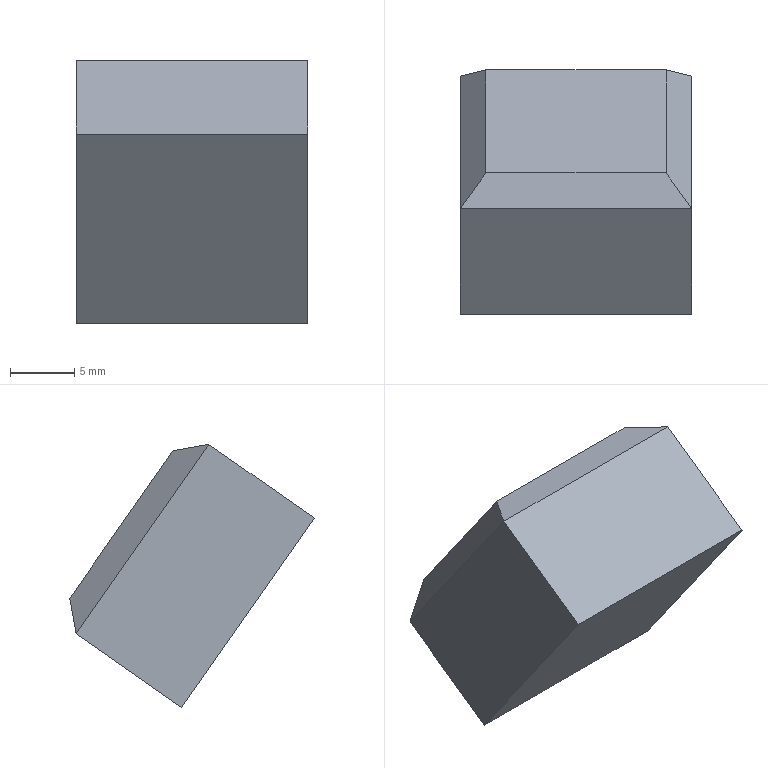Part | STEP file | Positioning_id1734_x_t | 1 solid | 10 faces | box 18 x 19.007 x 20.481 mm | volume 3755 mm3 | plane 10
STEP:
#1=CARTESIAN_POINT('',(0.,0.,0.));
#2=DIRECTION('',(0.,0.,1.));
#3=DIRECTION('',(1.,0.,0.));
#4=AXIS2_PLACEMENT_3D('',#1,#2,#3);
#5=CARTESIAN_POINT('',(-644.002,380.573,408.265));
#6=VERTEX_POINT('',#5);
#7=CARTESIAN_POINT('',(-646.002,380.082,405.48));
#8=VERTEX_POINT('',#7);
#9=CARTESIAN_POINT('',(-644.002,380.573,408.265));
#10=DIRECTION('',(-0.5774,-0.1418,-0.8041));
#11=VECTOR('',#10,1.);
#12=LINE('',#9,#11);
#13=CARTESIAN_POINT('',(-637.002,380.573,408.265));
#14=DIRECTION('',(0.,-0.9848,0.1736));
#15=DIRECTION('',(0.,-0.1736,-0.9848));
#16=AXIS2_PLACEMENT_3D('',#13,#14,#15);
#17=PLANE('',#16);
#18=CARTESIAN_POINT('',(0.,-7.));
#19=DIRECTION('',(0.8165,-0.5774));
#20=VECTOR('',#19,1.);
#21=LINE('',#18,#20);
#22=(GEOMETRIC_REPRESENTATION_CONTEXT(2)PARAMETRIC_REPRESENTATION_CONTEXT()REPRESENTATION_CONTEXT('',''));
#23=DEFINITIONAL_REPRESENTATION('',(#21),#22);
#24=PCURVE('',#17,#23);
#25=CARTESIAN_POINT('',(-644.002,376.558,413.999));
#26=DIRECTION('',(0.7071,-0.5792,-0.4056));
#27=DIRECTION('',(0.7071,0.5792,0.4056));
#28=AXIS2_PLACEMENT_3D('',#25,#26,#27);
#29=PLANE('',#28);
#30=CARTESIAN_POINT('',(0.,-7.));
#31=DIRECTION('',(-0.8165,-0.5774));
#32=VECTOR('',#31,1.);
#33=LINE('',#30,#32);
#34=(GEOMETRIC_REPRESENTATION_CONTEXT(2)PARAMETRIC_REPRESENTATION_CONTEXT()REPRESENTATION_CONTEXT('',''));
#35=DEFINITIONAL_REPRESENTATION('',(#33),#34);
#36=PCURVE('',#29,#35);
#37=SURFACE_CURVE('',#12,(#24,#36),.PCURVE_S1.);
#38=EDGE_CURVE('',#6,#8,#37,.T.);
#39=ORIENTED_EDGE('',*,*,#38,.F.);
#40=CARTESIAN_POINT('',(-630.002,380.573,408.265));
#41=VERTEX_POINT('',#40);
#42=CARTESIAN_POINT('',(-644.002,380.573,408.265));
#43=DIRECTION('',(1.,0.,0.));
#44=VECTOR('',#43,1.);
#45=LINE('',#42,#44);
#46=CARTESIAN_POINT('',(0.,-7.));
#47=DIRECTION('',(0.,1.));
#48=VECTOR('',#47,1.);
#49=LINE('',#46,#48);
#50=(GEOMETRIC_REPRESENTATION_CONTEXT(2)PARAMETRIC_REPRESENTATION_CONTEXT()REPRESENTATION_CONTEXT('',''));
#51=DEFINITIONAL_REPRESENTATION('',(#49),#50);
#52=PCURVE('',#17,#51);
#53=CARTESIAN_POINT('',(-637.002,376.558,413.999));
#54=DIRECTION('',(0.,0.8192,0.5736));
#55=DIRECTION('',(1.,0.,0.));
#56=AXIS2_PLACEMENT_3D('',#53,#54,#55);
#57=PLANE('',#56);
#58=CARTESIAN_POINT('',(-7.,7.));
#59=DIRECTION('',(1.,0.));
#60=VECTOR('',#59,1.);
#61=LINE('',#58,#60);
#62=(GEOMETRIC_REPRESENTATION_CONTEXT(2)PARAMETRIC_REPRESENTATION_CONTEXT()REPRESENTATION_CONTEXT('',''));
#63=DEFINITIONAL_REPRESENTATION('',(#61),#62);
#64=PCURVE('',#57,#63);
#65=SURFACE_CURVE('',#45,(#52,#64),.PCURVE_S1.);
#66=EDGE_CURVE('',#6,#41,#65,.T.);
#67=ORIENTED_EDGE('',*,*,#66,.T.);
#68=CARTESIAN_POINT('',(-628.002,380.082,405.48));
#69=VERTEX_POINT('',#68);
#70=CARTESIAN_POINT('',(-628.002,380.082,405.48));
#71=DIRECTION('',(-0.5774,0.1418,0.8041));
#72=VECTOR('',#71,1.);
#73=LINE('',#70,#72);
#74=CARTESIAN_POINT('',(2.828,9.));
#75=DIRECTION('',(-0.8165,-0.5774));
#76=VECTOR('',#75,1.);
#77=LINE('',#74,#76);
#78=(GEOMETRIC_REPRESENTATION_CONTEXT(2)PARAMETRIC_REPRESENTATION_CONTEXT()REPRESENTATION_CONTEXT('',''));
#79=DEFINITIONAL_REPRESENTATION('',(#77),#78);
#80=PCURVE('',#17,#79);
#81=CARTESIAN_POINT('',(-630.002,376.558,413.999));
#82=DIRECTION('',(-0.7071,-0.5792,-0.4056));
#83=DIRECTION('',(0.7071,-0.5792,-0.4056));
#84=AXIS2_PLACEMENT_3D('',#81,#82,#83);
#85=PLANE('',#84);
#86=CARTESIAN_POINT('',(2.828,-9.));
#87=DIRECTION('',(-0.8165,0.5774));
#88=VECTOR('',#87,1.);
#89=LINE('',#86,#88);
#90=(GEOMETRIC_REPRESENTATION_CONTEXT(2)PARAMETRIC_REPRESENTATION_CONTEXT()REPRESENTATION_CONTEXT('',''));
#91=DEFINITIONAL_REPRESENTATION('',(#89),#90);
#92=PCURVE('',#85,#91);
#93=SURFACE_CURVE('',#73,(#80,#92),.PCURVE_S1.);
#94=EDGE_CURVE('',#69,#41,#93,.T.);
#95=ORIENTED_EDGE('',*,*,#94,.F.);
#96=CARTESIAN_POINT('',(-628.002,380.082,405.48));
#97=DIRECTION('',(-1.,0.,0.));
#98=VECTOR('',#97,1.);
#99=LINE('',#96,#98);
#100=CARTESIAN_POINT('',(2.828,9.));
#101=DIRECTION('',(0.,-1.));
#102=VECTOR('',#101,1.);
#103=LINE('',#100,#102);
#104=(GEOMETRIC_REPRESENTATION_CONTEXT(2)PARAMETRIC_REPRESENTATION_CONTEXT()REPRESENTATION_CONTEXT('',''));
#105=DEFINITIONAL_REPRESENTATION('',(#103),#104);
#106=PCURVE('',#17,#105);
#107=CARTESIAN_POINT('',(-637.002,381.721,406.627));
#108=DIRECTION('',(0.,0.5736,-0.8192));
#109=DIRECTION('',(0.,-0.8192,-0.5736));
#110=AXIS2_PLACEMENT_3D('',#107,#108,#109);
#111=PLANE('',#110);
#112=CARTESIAN_POINT('',(2.,-9.));
#113=DIRECTION('',(0.,1.));
#114=VECTOR('',#113,1.);
#115=LINE('',#112,#114);
#116=(GEOMETRIC_REPRESENTATION_CONTEXT(2)PARAMETRIC_REPRESENTATION_CONTEXT()REPRESENTATION_CONTEXT('',''));
#117=DEFINITIONAL_REPRESENTATION('',(#115),#116);
#118=PCURVE('',#111,#117);
#119=SURFACE_CURVE('',#99,(#106,#118),.PCURVE_S1.);
#120=EDGE_CURVE('',#69,#8,#119,.T.);
#121=ORIENTED_EDGE('',*,*,#120,.T.);
#122=EDGE_LOOP('',(#39,#67,#95,#121));
#123=FACE_BOUND('',#122,.T.);
#124=ADVANCED_FACE('',(#123),#17,.F.);
#125=CARTESIAN_POINT('',(-628.002,369.758,420.225));
#126=VERTEX_POINT('',#125);
#127=CARTESIAN_POINT('',(-630.002,372.543,419.734));
#128=VERTEX_POINT('',#127);
#129=CARTESIAN_POINT('',(-628.002,369.758,420.225));
#130=DIRECTION('',(-0.5774,0.8041,-0.1418));
#131=VECTOR('',#130,1.);
#132=LINE('',#129,#131);
#133=CARTESIAN_POINT('',(2.828,9.));
#134=DIRECTION('',(-0.8165,-0.5774));
#135=VECTOR('',#134,1.);
#136=LINE('',#133,#135);
#137=(GEOMETRIC_REPRESENTATION_CONTEXT(2)PARAMETRIC_REPRESENTATION_CONTEXT()REPRESENTATION_CONTEXT('',''));
#138=DEFINITIONAL_REPRESENTATION('',(#136),#137);
#139=PCURVE('',#85,#138);
#140=CARTESIAN_POINT('',(-637.002,372.543,419.734));
#141=DIRECTION('',(0.,-0.1736,-0.9848));
#142=DIRECTION('',(0.,0.9848,-0.1736));
#143=AXIS2_PLACEMENT_3D('',#140,#141,#142);
#144=PLANE('',#143);
#145=CARTESIAN_POINT('',(-2.828,9.));
#146=DIRECTION('',(0.8165,-0.5774));
#147=VECTOR('',#146,1.);
#148=LINE('',#145,#147);
#149=(GEOMETRIC_REPRESENTATION_CONTEXT(2)PARAMETRIC_REPRESENTATION_CONTEXT()REPRESENTATION_CONTEXT('',''));
#150=DEFINITIONAL_REPRESENTATION('',(#148),#149);
#151=PCURVE('',#144,#150);
#152=SURFACE_CURVE('',#132,(#139,#151),.PCURVE_S1.);
#153=EDGE_CURVE('',#126,#128,#152,.T.);
#154=ORIENTED_EDGE('',*,*,#153,.F.);
#155=CARTESIAN_POINT('',(-628.002,369.758,420.225));
#156=DIRECTION('',(0.,0.5736,-0.8192));
#157=VECTOR('',#156,1.);
#158=LINE('',#155,#157);
#159=CARTESIAN_POINT('',(2.828,9.));
#160=DIRECTION('',(0.,-1.));
#161=VECTOR('',#160,1.);
#162=LINE('',#159,#161);
#163=(GEOMETRIC_REPRESENTATION_CONTEXT(2)PARAMETRIC_REPRESENTATION_CONTEXT()REPRESENTATION_CONTEXT('',''));
#164=DEFINITIONAL_REPRESENTATION('',(#162),#163);
#165=PCURVE('',#85,#164);
#166=CARTESIAN_POINT('',(-628.002,376.558,413.999));
#167=DIRECTION('',(1.,0.,0.));
#168=DIRECTION('',(0.,-0.8192,-0.5736));
#169=AXIS2_PLACEMENT_3D('',#166,#167,#168);
#170=PLANE('',#169);
#171=CARTESIAN_POINT('',(2.,-9.));
#172=DIRECTION('',(0.,1.));
#173=VECTOR('',#172,1.);
#174=LINE('',#171,#173);
#175=(GEOMETRIC_REPRESENTATION_CONTEXT(2)PARAMETRIC_REPRESENTATION_CONTEXT()REPRESENTATION_CONTEXT('',''));
#176=DEFINITIONAL_REPRESENTATION('',(#174),#175);
#177=PCURVE('',#170,#176);
#178=SURFACE_CURVE('',#158,(#165,#177),.PCURVE_S1.);
#179=EDGE_CURVE('',#126,#69,#178,.T.);
#180=ORIENTED_EDGE('',*,*,#179,.T.);
#181=ORIENTED_EDGE('',*,*,#94,.T.);
#182=CARTESIAN_POINT('',(-630.002,380.573,408.265));
#183=DIRECTION('',(0.,-0.5736,0.8192));
#184=VECTOR('',#183,1.);
#185=LINE('',#182,#184);
#186=CARTESIAN_POINT('',(0.,-7.));
#187=DIRECTION('',(0.,1.));
#188=VECTOR('',#187,1.);
#189=LINE('',#186,#188);
#190=(GEOMETRIC_REPRESENTATION_CONTEXT(2)PARAMETRIC_REPRESENTATION_CONTEXT()REPRESENTATION_CONTEXT('',''));
#191=DEFINITIONAL_REPRESENTATION('',(#189),#190);
#192=PCURVE('',#85,#191);
#193=CARTESIAN_POINT('',(7.,7.));
#194=DIRECTION('',(0.,-1.));
#195=VECTOR('',#194,1.);
#196=LINE('',#193,#195);
#197=(GEOMETRIC_REPRESENTATION_CONTEXT(2)PARAMETRIC_REPRESENTATION_CONTEXT()REPRESENTATION_CONTEXT('',''));
#198=DEFINITIONAL_REPRESENTATION('',(#196),#197);
#199=PCURVE('',#57,#198);
#200=SURFACE_CURVE('',#185,(#192,#199),.PCURVE_S1.);
#201=EDGE_CURVE('',#41,#128,#200,.T.);
#202=ORIENTED_EDGE('',*,*,#201,.T.);
#203=EDGE_LOOP('',(#154,#180,#181,#202));
#204=FACE_BOUND('',#203,.T.);
#205=ADVANCED_FACE('',(#204),#85,.F.);
#206=CARTESIAN_POINT('',(-644.002,372.543,419.734));
#207=VERTEX_POINT('',#206);
#208=CARTESIAN_POINT('',(-646.002,369.758,420.225));
#209=VERTEX_POINT('',#208);
#210=CARTESIAN_POINT('',(-644.002,372.543,419.734));
#211=DIRECTION('',(-0.5774,-0.8041,0.1418));
#212=VECTOR('',#211,1.);
#213=LINE('',#210,#212);
#214=CARTESIAN_POINT('',(0.,7.));
#215=DIRECTION('',(-0.8165,0.5774));
#216=VECTOR('',#215,1.);
#217=LINE('',#214,#216);
#218=(GEOMETRIC_REPRESENTATION_CONTEXT(2)PARAMETRIC_REPRESENTATION_CONTEXT()REPRESENTATION_CONTEXT('',''));
#219=DEFINITIONAL_REPRESENTATION('',(#217),#218);
#220=PCURVE('',#29,#219);
#221=CARTESIAN_POINT('',(0.,-7.));
#222=DIRECTION('',(-0.8165,-0.5774));
#223=VECTOR('',#222,1.);
#224=LINE('',#221,#223);
#225=(GEOMETRIC_REPRESENTATION_CONTEXT(2)PARAMETRIC_REPRESENTATION_CONTEXT()REPRESENTATION_CONTEXT('',''));
#226=DEFINITIONAL_REPRESENTATION('',(#224),#225);
#227=PCURVE('',#144,#226);
#228=SURFACE_CURVE('',#213,(#220,#227),.PCURVE_S1.);
#229=EDGE_CURVE('',#207,#209,#228,.T.);
#230=ORIENTED_EDGE('',*,*,#229,.F.);
#231=CARTESIAN_POINT('',(-644.002,372.543,419.734));
#232=DIRECTION('',(0.,0.5736,-0.8192));
#233=VECTOR('',#232,1.);
#234=LINE('',#231,#233);
#235=CARTESIAN_POINT('',(0.,7.));
#236=DIRECTION('',(0.,-1.));
#237=VECTOR('',#236,1.);
#238=LINE('',#235,#237);
#239=(GEOMETRIC_REPRESENTATION_CONTEXT(2)PARAMETRIC_REPRESENTATION_CONTEXT()REPRESENTATION_CONTEXT('',''));
#240=DEFINITIONAL_REPRESENTATION('',(#238),#239);
#241=PCURVE('',#29,#240);
#242=CARTESIAN_POINT('',(-7.,-7.));
#243=DIRECTION('',(0.,1.));
#244=VECTOR('',#243,1.);
#245=LINE('',#242,#244);
#246=(GEOMETRIC_REPRESENTATION_CONTEXT(2)PARAMETRIC_REPRESENTATION_CONTEXT()REPRESENTATION_CONTEXT('',''));
#247=DEFINITIONAL_REPRESENTATION('',(#245),#246);
#248=PCURVE('',#57,#247);
#249=SURFACE_CURVE('',#234,(#241,#248),.PCURVE_S1.);
#250=EDGE_CURVE('',#207,#6,#249,.T.);
#251=ORIENTED_EDGE('',*,*,#250,.T.);
#252=ORIENTED_EDGE('',*,*,#38,.T.);
#253=CARTESIAN_POINT('',(-646.002,380.082,405.48));
#254=DIRECTION('',(0.,-0.5736,0.8192));
#255=VECTOR('',#254,1.);
#256=LINE('',#253,#255);
#257=CARTESIAN_POINT('',(-2.828,-9.));
#258=DIRECTION('',(0.,1.));
#259=VECTOR('',#258,1.);
#260=LINE('',#257,#259);
#261=(GEOMETRIC_REPRESENTATION_CONTEXT(2)PARAMETRIC_REPRESENTATION_CONTEXT()REPRESENTATION_CONTEXT('',''));
#262=DEFINITIONAL_REPRESENTATION('',(#260),#261);
#263=PCURVE('',#29,#262);
#264=CARTESIAN_POINT('',(-646.002,376.558,413.999));
#265=DIRECTION('',(-1.,0.,0.));
#266=DIRECTION('',(0.,0.8192,0.5736));
#267=AXIS2_PLACEMENT_3D('',#264,#265,#266);
#268=PLANE('',#267);
#269=CARTESIAN_POINT('',(-2.,9.));
#270=DIRECTION('',(0.,-1.));
#271=VECTOR('',#270,1.);
#272=LINE('',#269,#271);
#273=(GEOMETRIC_REPRESENTATION_CONTEXT(2)PARAMETRIC_REPRESENTATION_CONTEXT()REPRESENTATION_CONTEXT('',''));
#274=DEFINITIONAL_REPRESENTATION('',(#272),#273);
#275=PCURVE('',#268,#274);
#276=SURFACE_CURVE('',#256,(#263,#275),.PCURVE_S1.);
#277=EDGE_CURVE('',#8,#209,#276,.T.);
#278=ORIENTED_EDGE('',*,*,#277,.T.);
#279=EDGE_LOOP('',(#230,#251,#252,#278));
#280=FACE_BOUND('',#279,.T.);
#281=ADVANCED_FACE('',(#280),#29,.F.);
#282=ORIENTED_EDGE('',*,*,#153,.T.);
#283=CARTESIAN_POINT('',(-630.002,372.543,419.734));
#284=DIRECTION('',(-1.,0.,0.));
#285=VECTOR('',#284,1.);
#286=LINE('',#283,#285);
#287=CARTESIAN_POINT('',(0.,7.));
#288=DIRECTION('',(0.,-1.));
#289=VECTOR('',#288,1.);
#290=LINE('',#287,#289);
#291=(GEOMETRIC_REPRESENTATION_CONTEXT(2)PARAMETRIC_REPRESENTATION_CONTEXT()REPRESENTATION_CONTEXT('',''));
#292=DEFINITIONAL_REPRESENTATION('',(#290),#291);
#293=PCURVE('',#144,#292);
#294=CARTESIAN_POINT('',(7.,-7.));
#295=DIRECTION('',(-1.,0.));
#296=VECTOR('',#295,1.);
#297=LINE('',#294,#296);
#298=(GEOMETRIC_REPRESENTATION_CONTEXT(2)PARAMETRIC_REPRESENTATION_CONTEXT()REPRESENTATION_CONTEXT('',''));
#299=DEFINITIONAL_REPRESENTATION('',(#297),#298);
#300=PCURVE('',#57,#299);
#301=SURFACE_CURVE('',#286,(#293,#300),.PCURVE_S1.);
#302=EDGE_CURVE('',#128,#207,#301,.T.);
#303=ORIENTED_EDGE('',*,*,#302,.T.);
#304=ORIENTED_EDGE('',*,*,#229,.T.);
#305=CARTESIAN_POINT('',(-646.002,369.758,420.225));
#306=DIRECTION('',(1.,0.,0.));
#307=VECTOR('',#306,1.);
#308=LINE('',#305,#307);
#309=CARTESIAN_POINT('',(-2.828,-9.));
#310=DIRECTION('',(0.,1.));
#311=VECTOR('',#310,1.);
#312=LINE('',#309,#311);
#313=(GEOMETRIC_REPRESENTATION_CONTEXT(2)PARAMETRIC_REPRESENTATION_CONTEXT()REPRESENTATION_CONTEXT('',''));
#314=DEFINITIONAL_REPRESENTATION('',(#312),#313);
#315=PCURVE('',#144,#314);
#316=CARTESIAN_POINT('',(-637.002,371.396,421.372));
#317=DIRECTION('',(0.,-0.5736,0.8192));
#318=DIRECTION('',(0.,0.8192,0.5736));
#319=AXIS2_PLACEMENT_3D('',#316,#317,#318);
#320=PLANE('',#319);
#321=CARTESIAN_POINT('',(-2.,9.));
#322=DIRECTION('',(0.,-1.));
#323=VECTOR('',#322,1.);
#324=LINE('',#321,#323);
#325=(GEOMETRIC_REPRESENTATION_CONTEXT(2)PARAMETRIC_REPRESENTATION_CONTEXT()REPRESENTATION_CONTEXT('',''));
#326=DEFINITIONAL_REPRESENTATION('',(#324),#325);
#327=PCURVE('',#320,#326);
#328=SURFACE_CURVE('',#308,(#315,#327),.PCURVE_S1.);
#329=EDGE_CURVE('',#209,#126,#328,.T.);
#330=ORIENTED_EDGE('',*,*,#329,.T.);
#331=EDGE_LOOP('',(#282,#303,#304,#330));
#332=FACE_BOUND('',#331,.T.);
#333=ADVANCED_FACE('',(#332),#144,.F.);
#334=CARTESIAN_POINT('',(-628.002,361.566,414.489));
#335=VERTEX_POINT('',#334);
#336=CARTESIAN_POINT('',(-628.002,369.758,420.225));
#337=DIRECTION('',(0.,-0.8192,-0.5736));
#338=VECTOR('',#337,1.);
#339=LINE('',#336,#338);
#340=CARTESIAN_POINT('',(2.,-9.));
#341=DIRECTION('',(1.,0.));
#342=VECTOR('',#341,1.);
#343=LINE('',#340,#342);
#344=(GEOMETRIC_REPRESENTATION_CONTEXT(2)PARAMETRIC_REPRESENTATION_CONTEXT()REPRESENTATION_CONTEXT('',''));
#345=DEFINITIONAL_REPRESENTATION('',(#343),#344);
#346=PCURVE('',#170,#345);
#347=CARTESIAN_POINT('',(-2.,-9.));
#348=DIRECTION('',(-1.,0.));
#349=VECTOR('',#348,1.);
#350=LINE('',#347,#349);
#351=(GEOMETRIC_REPRESENTATION_CONTEXT(2)PARAMETRIC_REPRESENTATION_CONTEXT()REPRESENTATION_CONTEXT('',''));
#352=DEFINITIONAL_REPRESENTATION('',(#350),#351);
#353=PCURVE('',#320,#352);
#354=SURFACE_CURVE('',#339,(#346,#353),.PCURVE_S1.);
#355=EDGE_CURVE('',#126,#335,#354,.T.);
#356=ORIENTED_EDGE('',*,*,#355,.T.);
#357=CARTESIAN_POINT('',(-628.002,371.891,399.744));
#358=VERTEX_POINT('',#357);
#359=CARTESIAN_POINT('',(-628.002,361.566,414.489));
#360=DIRECTION('',(0.,0.5736,-0.8192));
#361=VECTOR('',#360,1.);
#362=LINE('',#359,#361);
#363=CARTESIAN_POINT('',(12.,-9.));
#364=DIRECTION('',(0.,1.));
#365=VECTOR('',#364,1.);
#366=LINE('',#363,#365);
#367=(GEOMETRIC_REPRESENTATION_CONTEXT(2)PARAMETRIC_REPRESENTATION_CONTEXT()REPRESENTATION_CONTEXT('',''));
#368=DEFINITIONAL_REPRESENTATION('',(#366),#367);
#369=PCURVE('',#170,#368);
#370=CARTESIAN_POINT('',(-637.002,366.729,407.117));
#371=DIRECTION('',(0.,-0.8192,-0.5736));
#372=DIRECTION('',(-1.,0.,0.));
#373=AXIS2_PLACEMENT_3D('',#370,#371,#372);
#374=PLANE('',#373);
#375=CARTESIAN_POINT('',(-9.,-9.));
#376=DIRECTION('',(0.,1.));
#377=VECTOR('',#376,1.);
#378=LINE('',#375,#377);
#379=(GEOMETRIC_REPRESENTATION_CONTEXT(2)PARAMETRIC_REPRESENTATION_CONTEXT()REPRESENTATION_CONTEXT('',''));
#380=DEFINITIONAL_REPRESENTATION('',(#378),#379);
#381=PCURVE('',#374,#380);
#382=SURFACE_CURVE('',#362,(#369,#381),.PCURVE_S1.);
#383=EDGE_CURVE('',#335,#358,#382,.T.);
#384=ORIENTED_EDGE('',*,*,#383,.T.);
#385=CARTESIAN_POINT('',(-628.002,380.082,405.48));
#386=DIRECTION('',(0.,-0.8192,-0.5736));
#387=VECTOR('',#386,1.);
#388=LINE('',#385,#387);
#389=CARTESIAN_POINT('',(2.,9.));
#390=DIRECTION('',(1.,0.));
#391=VECTOR('',#390,1.);
#392=LINE('',#389,#391);
#393=(GEOMETRIC_REPRESENTATION_CONTEXT(2)PARAMETRIC_REPRESENTATION_CONTEXT()REPRESENTATION_CONTEXT('',''));
#394=DEFINITIONAL_REPRESENTATION('',(#392),#393);
#395=PCURVE('',#170,#394);
#396=CARTESIAN_POINT('',(2.,-9.));
#397=DIRECTION('',(1.,0.));
#398=VECTOR('',#397,1.);
#399=LINE('',#396,#398);
#400=(GEOMETRIC_REPRESENTATION_CONTEXT(2)PARAMETRIC_REPRESENTATION_CONTEXT()REPRESENTATION_CONTEXT('',''));
#401=DEFINITIONAL_REPRESENTATION('',(#399),#400);
#402=PCURVE('',#111,#401);
#403=SURFACE_CURVE('',#388,(#395,#402),.PCURVE_S1.);
#404=EDGE_CURVE('',#69,#358,#403,.T.);
#405=ORIENTED_EDGE('',*,*,#404,.F.);
#406=ORIENTED_EDGE('',*,*,#179,.F.);
#407=EDGE_LOOP('',(#356,#384,#405,#406));
#408=FACE_BOUND('',#407,.T.);
#409=ADVANCED_FACE('',(#408),#170,.T.);
#410=ORIENTED_EDGE('',*,*,#250,.F.);
#411=ORIENTED_EDGE('',*,*,#302,.F.);
#412=ORIENTED_EDGE('',*,*,#201,.F.);
#413=ORIENTED_EDGE('',*,*,#66,.F.);
#414=EDGE_LOOP('',(#410,#411,#412,#413));
#415=FACE_BOUND('',#414,.T.);
#416=ADVANCED_FACE('',(#415),#57,.T.);
#417=CARTESIAN_POINT('',(-646.002,361.566,414.489));
#418=VERTEX_POINT('',#417);
#419=CARTESIAN_POINT('',(-646.002,369.758,420.225));
#420=DIRECTION('',(0.,-0.8192,-0.5736));
#421=VECTOR('',#420,1.);
#422=LINE('',#419,#421);
#423=CARTESIAN_POINT('',(-2.,9.));
#424=DIRECTION('',(-1.,0.));
#425=VECTOR('',#424,1.);
#426=LINE('',#423,#425);
#427=(GEOMETRIC_REPRESENTATION_CONTEXT(2)PARAMETRIC_REPRESENTATION_CONTEXT()REPRESENTATION_CONTEXT('',''));
#428=DEFINITIONAL_REPRESENTATION('',(#426),#427);
#429=PCURVE('',#320,#428);
#430=CARTESIAN_POINT('',(-2.,-9.));
#431=DIRECTION('',(-1.,0.));
#432=VECTOR('',#431,1.);
#433=LINE('',#430,#432);
#434=(GEOMETRIC_REPRESENTATION_CONTEXT(2)PARAMETRIC_REPRESENTATION_CONTEXT()REPRESENTATION_CONTEXT('',''));
#435=DEFINITIONAL_REPRESENTATION('',(#433),#434);
#436=PCURVE('',#268,#435);
#437=SURFACE_CURVE('',#422,(#429,#436),.PCURVE_S1.);
#438=EDGE_CURVE('',#209,#418,#437,.T.);
#439=ORIENTED_EDGE('',*,*,#438,.T.);
#440=CARTESIAN_POINT('',(-646.002,361.566,414.489));
#441=DIRECTION('',(1.,0.,0.));
#442=VECTOR('',#441,1.);
#443=LINE('',#440,#442);
#444=CARTESIAN_POINT('',(-12.,9.));
#445=DIRECTION('',(0.,-1.));
#446=VECTOR('',#445,1.);
#447=LINE('',#444,#446);
#448=(GEOMETRIC_REPRESENTATION_CONTEXT(2)PARAMETRIC_REPRESENTATION_CONTEXT()REPRESENTATION_CONTEXT('',''));
#449=DEFINITIONAL_REPRESENTATION('',(#447),#448);
#450=PCURVE('',#320,#449);
#451=CARTESIAN_POINT('',(9.,-9.));
#452=DIRECTION('',(-1.,0.));
#453=VECTOR('',#452,1.);
#454=LINE('',#451,#453);
#455=(GEOMETRIC_REPRESENTATION_CONTEXT(2)PARAMETRIC_REPRESENTATION_CONTEXT()REPRESENTATION_CONTEXT('',''));
#456=DEFINITIONAL_REPRESENTATION('',(#454),#455);
#457=PCURVE('',#374,#456);
#458=SURFACE_CURVE('',#443,(#450,#457),.PCURVE_S1.);
#459=EDGE_CURVE('',#418,#335,#458,.T.);
#460=ORIENTED_EDGE('',*,*,#459,.T.);
#461=ORIENTED_EDGE('',*,*,#355,.F.);
#462=ORIENTED_EDGE('',*,*,#329,.F.);
#463=EDGE_LOOP('',(#439,#460,#461,#462));
#464=FACE_BOUND('',#463,.T.);
#465=ADVANCED_FACE('',(#464),#320,.T.);
#466=CARTESIAN_POINT('',(-646.002,371.891,399.744));
#467=VERTEX_POINT('',#466);
#468=CARTESIAN_POINT('',(-646.002,380.082,405.48));
#469=DIRECTION('',(0.,-0.8192,-0.5736));
#470=VECTOR('',#469,1.);
#471=LINE('',#468,#470);
#472=CARTESIAN_POINT('',(-2.,9.));
#473=DIRECTION('',(-1.,0.));
#474=VECTOR('',#473,1.);
#475=LINE('',#472,#474);
#476=(GEOMETRIC_REPRESENTATION_CONTEXT(2)PARAMETRIC_REPRESENTATION_CONTEXT()REPRESENTATION_CONTEXT('',''));
#477=DEFINITIONAL_REPRESENTATION('',(#475),#476);
#478=PCURVE('',#268,#477);
#479=CARTESIAN_POINT('',(2.,9.));
#480=DIRECTION('',(1.,0.));
#481=VECTOR('',#480,1.);
#482=LINE('',#479,#481);
#483=(GEOMETRIC_REPRESENTATION_CONTEXT(2)PARAMETRIC_REPRESENTATION_CONTEXT()REPRESENTATION_CONTEXT('',''));
#484=DEFINITIONAL_REPRESENTATION('',(#482),#483);
#485=PCURVE('',#111,#484);
#486=SURFACE_CURVE('',#471,(#478,#485),.PCURVE_S1.);
#487=EDGE_CURVE('',#8,#467,#486,.T.);
#488=ORIENTED_EDGE('',*,*,#487,.T.);
#489=CARTESIAN_POINT('',(-646.002,371.891,399.744));
#490=DIRECTION('',(0.,-0.5736,0.8192));
#491=VECTOR('',#490,1.);
#492=LINE('',#489,#491);
#493=CARTESIAN_POINT('',(-12.,9.));
#494=DIRECTION('',(0.,-1.));
#495=VECTOR('',#494,1.);
#496=LINE('',#493,#495);
#497=(GEOMETRIC_REPRESENTATION_CONTEXT(2)PARAMETRIC_REPRESENTATION_CONTEXT()REPRESENTATION_CONTEXT('',''));
#498=DEFINITIONAL_REPRESENTATION('',(#496),#497);
#499=PCURVE('',#268,#498);
#500=CARTESIAN_POINT('',(9.,9.));
#501=DIRECTION('',(0.,-1.));
#502=VECTOR('',#501,1.);
#503=LINE('',#500,#502);
#504=(GEOMETRIC_REPRESENTATION_CONTEXT(2)PARAMETRIC_REPRESENTATION_CONTEXT()REPRESENTATION_CONTEXT('',''));
#505=DEFINITIONAL_REPRESENTATION('',(#503),#504);
#506=PCURVE('',#374,#505);
#507=SURFACE_CURVE('',#492,(#499,#506),.PCURVE_S1.);
#508=EDGE_CURVE('',#467,#418,#507,.T.);
#509=ORIENTED_EDGE('',*,*,#508,.T.);
#510=ORIENTED_EDGE('',*,*,#438,.F.);
#511=ORIENTED_EDGE('',*,*,#277,.F.);
#512=EDGE_LOOP('',(#488,#509,#510,#511));
#513=FACE_BOUND('',#512,.T.);
#514=ADVANCED_FACE('',(#513),#268,.T.);
#515=ORIENTED_EDGE('',*,*,#404,.T.);
#516=CARTESIAN_POINT('',(-628.002,371.891,399.744));
#517=DIRECTION('',(-1.,0.,0.));
#518=VECTOR('',#517,1.);
#519=LINE('',#516,#518);
#520=CARTESIAN_POINT('',(12.,-9.));
#521=DIRECTION('',(0.,1.));
#522=VECTOR('',#521,1.);
#523=LINE('',#520,#522);
#524=(GEOMETRIC_REPRESENTATION_CONTEXT(2)PARAMETRIC_REPRESENTATION_CONTEXT()REPRESENTATION_CONTEXT('',''));
#525=DEFINITIONAL_REPRESENTATION('',(#523),#524);
#526=PCURVE('',#111,#525);
#527=CARTESIAN_POINT('',(-9.,9.));
#528=DIRECTION('',(1.,0.));
#529=VECTOR('',#528,1.);
#530=LINE('',#527,#529);
#531=(GEOMETRIC_REPRESENTATION_CONTEXT(2)PARAMETRIC_REPRESENTATION_CONTEXT()REPRESENTATION_CONTEXT('',''));
#532=DEFINITIONAL_REPRESENTATION('',(#530),#531);
#533=PCURVE('',#374,#532);
#534=SURFACE_CURVE('',#519,(#526,#533),.PCURVE_S1.);
#535=EDGE_CURVE('',#358,#467,#534,.T.);
#536=ORIENTED_EDGE('',*,*,#535,.T.);
#537=ORIENTED_EDGE('',*,*,#487,.F.);
#538=ORIENTED_EDGE('',*,*,#120,.F.);
#539=EDGE_LOOP('',(#515,#536,#537,#538));
#540=FACE_BOUND('',#539,.T.);
#541=ADVANCED_FACE('',(#540),#111,.T.);
#542=ORIENTED_EDGE('',*,*,#535,.F.);
#543=ORIENTED_EDGE('',*,*,#383,.F.);
#544=ORIENTED_EDGE('',*,*,#459,.F.);
#545=ORIENTED_EDGE('',*,*,#508,.F.);
#546=EDGE_LOOP('',(#542,#543,#544,#545));
#547=FACE_BOUND('',#546,.T.);
#548=ADVANCED_FACE('',(#547),#374,.T.);
#549=CLOSED_SHELL('',(#124,#205,#281,#333,#409,#416,#465,#514,#541,#548));
#550=MANIFOLD_SOLID_BREP('',#549);
#551=(LENGTH_UNIT()NAMED_UNIT(*)SI_UNIT(.MILLI.,.METRE.));
#552=UNCERTAINTY_MEASURE_WITH_UNIT(LENGTH_MEASURE(0.0000001),#551,'','');
#553=(NAMED_UNIT(*)PLANE_ANGLE_UNIT()SI_UNIT($,.RADIAN.));
#554=(NAMED_UNIT(*)SI_UNIT($,.STERADIAN.)SOLID_ANGLE_UNIT());
#555=(GEOMETRIC_REPRESENTATION_CONTEXT(3)GLOBAL_UNCERTAINTY_ASSIGNED_CONTEXT((#552))GLOBAL_UNIT_ASSIGNED_CONTEXT((#551,#553,#554))REPRESENTATION_CONTEXT('',''));
#556=ADVANCED_BREP_SHAPE_REPRESENTATION('',(#4,#550),#555);